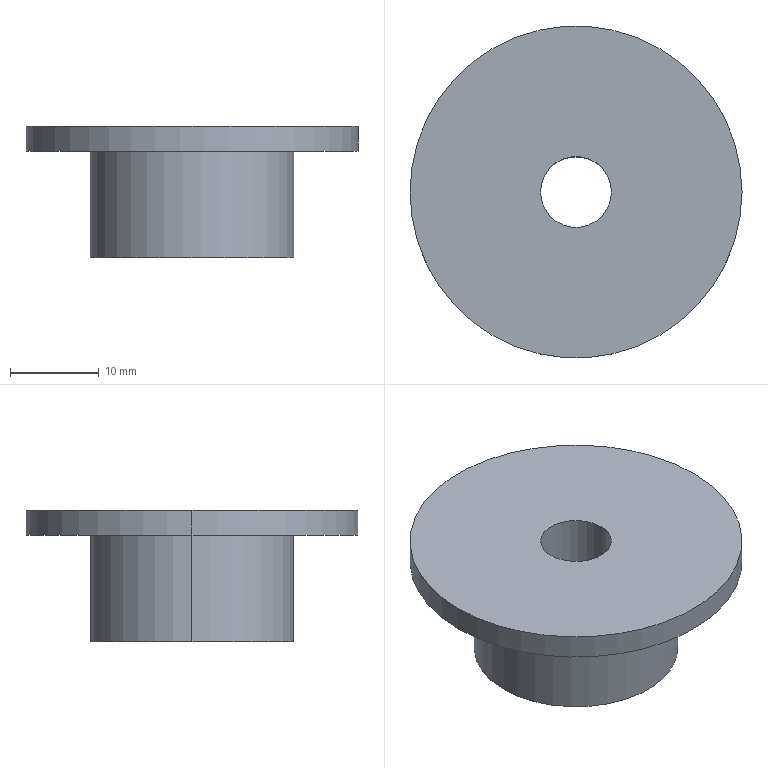Part | SolidWorks | features Extrusion 1, ICE 1 | 1 solid | 9 faces | box 37.5 x 37.5 x 14.8 mm | volume 7334 mm3 | cylinder 6 | plane 3 | commonest cylinder face diameters 8 x2 23 x2 37.5 x2
STEP:
#1=CARTESIAN_POINT('',(18.75,0.,14.8));
#2=VERTEX_POINT('',#1);
#3=CARTESIAN_POINT('',(-18.75,0.,14.8));
#4=VERTEX_POINT('',#3);
#5=CARTESIAN_POINT('',(0.,0.,14.8));
#6=DIRECTION('',(0.,0.,1.));
#7=DIRECTION('',(1.,0.,0.));
#8=AXIS2_PLACEMENT_3D('',#5,#6,#7);
#9=CIRCLE('',#8,18.75);
#10=EDGE_CURVE('',#2,#4,#9,.T.);
#11=ORIENTED_EDGE('',*,*,#10,.F.);
#12=CARTESIAN_POINT('',(18.75,0.,12.));
#13=VERTEX_POINT('',#12);
#14=CARTESIAN_POINT('',(18.75,0.,14.8));
#15=DIRECTION('',(0.,0.,-1.));
#16=VECTOR('',#15,1000.);
#17=LINE('',#14,#16);
#18=EDGE_CURVE('',#2,#13,#17,.T.);
#19=ORIENTED_EDGE('',*,*,#18,.T.);
#20=CARTESIAN_POINT('',(-18.75,0.,12.));
#21=VERTEX_POINT('',#20);
#22=CARTESIAN_POINT('',(0.,0.,12.));
#23=DIRECTION('',(0.,0.,1.));
#24=DIRECTION('',(1.,0.,0.));
#25=AXIS2_PLACEMENT_3D('',#22,#23,#24);
#26=CIRCLE('',#25,18.75);
#27=EDGE_CURVE('',#13,#21,#26,.T.);
#28=ORIENTED_EDGE('',*,*,#27,.T.);
#29=CARTESIAN_POINT('',(-18.75,0.,14.8));
#30=DIRECTION('',(0.,0.,-1.));
#31=VECTOR('',#30,1000.);
#32=LINE('',#29,#31);
#33=EDGE_CURVE('',#4,#21,#32,.T.);
#34=ORIENTED_EDGE('',*,*,#33,.F.);
#35=EDGE_LOOP('',(#11,#19,#28,#34));
#36=FACE_OUTER_BOUND('',#35,.T.);
#37=CARTESIAN_POINT('',(0.,0.,14.8));
#38=DIRECTION('',(0.,0.,-1.));
#39=DIRECTION('',(-1.,0.,0.));
#40=AXIS2_PLACEMENT_3D('',#37,#38,#39);
#41=CYLINDRICAL_SURFACE('',#40,18.75);
#42=ADVANCED_FACE('',(#36),#41,.T.);
#43=CARTESIAN_POINT('',(-4.,0.,14.8));
#44=VERTEX_POINT('',#43);
#45=CARTESIAN_POINT('',(4.,0.,14.8));
#46=VERTEX_POINT('',#45);
#47=CARTESIAN_POINT('',(0.,0.,14.8));
#48=DIRECTION('',(0.,0.,1.));
#49=DIRECTION('',(1.,0.,0.));
#50=AXIS2_PLACEMENT_3D('',#47,#48,#49);
#51=CIRCLE('',#50,4.);
#52=EDGE_CURVE('',#44,#46,#51,.T.);
#53=ORIENTED_EDGE('',*,*,#52,.T.);
#54=CARTESIAN_POINT('',(4.,0.,0.));
#55=VERTEX_POINT('',#54);
#56=CARTESIAN_POINT('',(4.,0.,12.));
#57=DIRECTION('',(0.,0.,-1.));
#58=VECTOR('',#57,1000.);
#59=LINE('',#56,#58);
#60=EDGE_CURVE('',#46,#55,#59,.T.);
#61=ORIENTED_EDGE('',*,*,#60,.T.);
#62=CARTESIAN_POINT('',(-4.,0.,0.));
#63=VERTEX_POINT('',#62);
#64=CARTESIAN_POINT('',(0.,0.,0.));
#65=DIRECTION('',(0.,0.,1.));
#66=DIRECTION('',(1.,0.,0.));
#67=AXIS2_PLACEMENT_3D('',#64,#65,#66);
#68=CIRCLE('',#67,4.);
#69=EDGE_CURVE('',#63,#55,#68,.T.);
#70=ORIENTED_EDGE('',*,*,#69,.F.);
#71=CARTESIAN_POINT('',(-4.,0.,12.));
#72=DIRECTION('',(0.,0.,-1.));
#73=VECTOR('',#72,1000.);
#74=LINE('',#71,#73);
#75=EDGE_CURVE('',#44,#63,#74,.T.);
#76=ORIENTED_EDGE('',*,*,#75,.F.);
#77=EDGE_LOOP('',(#53,#61,#70,#76));
#78=FACE_OUTER_BOUND('',#77,.T.);
#79=CARTESIAN_POINT('',(0.,0.,12.));
#80=DIRECTION('',(0.,0.,-1.));
#81=DIRECTION('',(-1.,0.,0.));
#82=AXIS2_PLACEMENT_3D('',#79,#80,#81);
#83=CYLINDRICAL_SURFACE('',#82,4.);
#84=ADVANCED_FACE('',(#78),#83,.F.);
#85=CARTESIAN_POINT('',(11.5,0.,12.));
#86=VERTEX_POINT('',#85);
#87=CARTESIAN_POINT('',(-11.5,0.,12.));
#88=VERTEX_POINT('',#87);
#89=CARTESIAN_POINT('',(0.,0.,12.));
#90=DIRECTION('',(0.,0.,1.));
#91=DIRECTION('',(1.,0.,0.));
#92=AXIS2_PLACEMENT_3D('',#89,#90,#91);
#93=CIRCLE('',#92,11.5);
#94=EDGE_CURVE('',#86,#88,#93,.T.);
#95=ORIENTED_EDGE('',*,*,#94,.F.);
#96=CARTESIAN_POINT('',(11.5,0.,0.));
#97=VERTEX_POINT('',#96);
#98=CARTESIAN_POINT('',(11.5,0.,12.));
#99=DIRECTION('',(0.,0.,-1.));
#100=VECTOR('',#99,1000.);
#101=LINE('',#98,#100);
#102=EDGE_CURVE('',#86,#97,#101,.T.);
#103=ORIENTED_EDGE('',*,*,#102,.T.);
#104=CARTESIAN_POINT('',(-11.5,0.,0.));
#105=VERTEX_POINT('',#104);
#106=CARTESIAN_POINT('',(0.,0.,0.));
#107=DIRECTION('',(0.,0.,1.));
#108=DIRECTION('',(1.,0.,0.));
#109=AXIS2_PLACEMENT_3D('',#106,#107,#108);
#110=CIRCLE('',#109,11.5);
#111=EDGE_CURVE('',#97,#105,#110,.T.);
#112=ORIENTED_EDGE('',*,*,#111,.T.);
#113=CARTESIAN_POINT('',(-11.5,0.,12.));
#114=DIRECTION('',(0.,0.,-1.));
#115=VECTOR('',#114,1000.);
#116=LINE('',#113,#115);
#117=EDGE_CURVE('',#88,#105,#116,.T.);
#118=ORIENTED_EDGE('',*,*,#117,.F.);
#119=EDGE_LOOP('',(#95,#103,#112,#118));
#120=FACE_OUTER_BOUND('',#119,.T.);
#121=CARTESIAN_POINT('',(0.,0.,12.));
#122=DIRECTION('',(0.,0.,-1.));
#123=DIRECTION('',(-1.,0.,0.));
#124=AXIS2_PLACEMENT_3D('',#121,#122,#123);
#125=CYLINDRICAL_SURFACE('',#124,11.5);
#126=ADVANCED_FACE('',(#120),#125,.T.);
#127=CARTESIAN_POINT('',(0.,0.,0.));
#128=DIRECTION('',(0.,0.,1.));
#129=DIRECTION('',(1.,0.,0.));
#130=AXIS2_PLACEMENT_3D('',#127,#128,#129);
#131=CIRCLE('',#130,11.5);
#132=EDGE_CURVE('',#105,#97,#131,.T.);
#133=ORIENTED_EDGE('',*,*,#132,.F.);
#134=ORIENTED_EDGE('',*,*,#111,.F.);
#135=EDGE_LOOP('',(#133,#134));
#136=FACE_OUTER_BOUND('',#135,.T.);
#137=ORIENTED_EDGE('',*,*,#69,.T.);
#138=CARTESIAN_POINT('',(0.,0.,0.));
#139=DIRECTION('',(0.,0.,1.));
#140=DIRECTION('',(1.,0.,0.));
#141=AXIS2_PLACEMENT_3D('',#138,#139,#140);
#142=CIRCLE('',#141,4.);
#143=EDGE_CURVE('',#55,#63,#142,.T.);
#144=ORIENTED_EDGE('',*,*,#143,.T.);
#145=EDGE_LOOP('',(#137,#144));
#146=FACE_BOUND('',#145,.T.);
#147=CARTESIAN_POINT('',(0.,0.,0.));
#148=DIRECTION('',(0.,0.,1.));
#149=DIRECTION('',(1.,0.,0.));
#150=AXIS2_PLACEMENT_3D('',#147,#148,#149);
#151=PLANE('',#150);
#152=ADVANCED_FACE('',(#136,#146),#151,.F.);
#153=ORIENTED_EDGE('',*,*,#102,.F.);
#154=CARTESIAN_POINT('',(0.,0.,12.));
#155=DIRECTION('',(0.,0.,1.));
#156=DIRECTION('',(1.,0.,0.));
#157=AXIS2_PLACEMENT_3D('',#154,#155,#156);
#158=CIRCLE('',#157,11.5);
#159=EDGE_CURVE('',#88,#86,#158,.T.);
#160=ORIENTED_EDGE('',*,*,#159,.F.);
#161=ORIENTED_EDGE('',*,*,#117,.T.);
#162=ORIENTED_EDGE('',*,*,#132,.T.);
#163=EDGE_LOOP('',(#153,#160,#161,#162));
#164=FACE_OUTER_BOUND('',#163,.T.);
#165=CARTESIAN_POINT('',(0.,0.,12.));
#166=DIRECTION('',(0.,0.,-1.));
#167=DIRECTION('',(-1.,0.,0.));
#168=AXIS2_PLACEMENT_3D('',#165,#166,#167);
#169=CYLINDRICAL_SURFACE('',#168,11.5);
#170=ADVANCED_FACE('',(#164),#169,.T.);
#171=ORIENTED_EDGE('',*,*,#60,.F.);
#172=CARTESIAN_POINT('',(0.,0.,14.8));
#173=DIRECTION('',(0.,0.,1.));
#174=DIRECTION('',(1.,0.,0.));
#175=AXIS2_PLACEMENT_3D('',#172,#173,#174);
#176=CIRCLE('',#175,4.);
#177=EDGE_CURVE('',#46,#44,#176,.T.);
#178=ORIENTED_EDGE('',*,*,#177,.T.);
#179=ORIENTED_EDGE('',*,*,#75,.T.);
#180=ORIENTED_EDGE('',*,*,#143,.F.);
#181=EDGE_LOOP('',(#171,#178,#179,#180));
#182=FACE_OUTER_BOUND('',#181,.T.);
#183=CARTESIAN_POINT('',(0.,0.,12.));
#184=DIRECTION('',(0.,0.,-1.));
#185=DIRECTION('',(-1.,0.,0.));
#186=AXIS2_PLACEMENT_3D('',#183,#184,#185);
#187=CYLINDRICAL_SURFACE('',#186,4.);
#188=ADVANCED_FACE('',(#182),#187,.F.);
#189=CARTESIAN_POINT('',(0.,0.,12.));
#190=DIRECTION('',(0.,0.,1.));
#191=DIRECTION('',(1.,0.,0.));
#192=AXIS2_PLACEMENT_3D('',#189,#190,#191);
#193=CIRCLE('',#192,18.75);
#194=EDGE_CURVE('',#21,#13,#193,.T.);
#195=ORIENTED_EDGE('',*,*,#194,.F.);
#196=ORIENTED_EDGE('',*,*,#27,.F.);
#197=EDGE_LOOP('',(#195,#196));
#198=FACE_OUTER_BOUND('',#197,.T.);
#199=ORIENTED_EDGE('',*,*,#159,.T.);
#200=ORIENTED_EDGE('',*,*,#94,.T.);
#201=EDGE_LOOP('',(#199,#200));
#202=FACE_BOUND('',#201,.T.);
#203=CARTESIAN_POINT('',(0.,0.,12.));
#204=DIRECTION('',(0.,0.,1.));
#205=DIRECTION('',(1.,0.,0.));
#206=AXIS2_PLACEMENT_3D('',#203,#204,#205);
#207=PLANE('',#206);
#208=ADVANCED_FACE('',(#198,#202),#207,.F.);
#209=CARTESIAN_POINT('',(0.,0.,14.8));
#210=DIRECTION('',(0.,0.,1.));
#211=DIRECTION('',(1.,0.,0.));
#212=AXIS2_PLACEMENT_3D('',#209,#210,#211);
#213=CIRCLE('',#212,18.75);
#214=EDGE_CURVE('',#4,#2,#213,.T.);
#215=ORIENTED_EDGE('',*,*,#214,.T.);
#216=ORIENTED_EDGE('',*,*,#10,.T.);
#217=EDGE_LOOP('',(#215,#216));
#218=FACE_OUTER_BOUND('',#217,.T.);
#219=ORIENTED_EDGE('',*,*,#52,.F.);
#220=ORIENTED_EDGE('',*,*,#177,.F.);
#221=EDGE_LOOP('',(#219,#220));
#222=FACE_BOUND('',#221,.T.);
#223=CARTESIAN_POINT('',(0.,0.,14.8));
#224=DIRECTION('',(0.,0.,1.));
#225=DIRECTION('',(1.,0.,0.));
#226=AXIS2_PLACEMENT_3D('',#223,#224,#225);
#227=PLANE('',#226);
#228=ADVANCED_FACE('',(#218,#222),#227,.T.);
#229=ORIENTED_EDGE('',*,*,#18,.F.);
#230=ORIENTED_EDGE('',*,*,#214,.F.);
#231=ORIENTED_EDGE('',*,*,#33,.T.);
#232=ORIENTED_EDGE('',*,*,#194,.T.);
#233=EDGE_LOOP('',(#229,#230,#231,#232));
#234=FACE_OUTER_BOUND('',#233,.T.);
#235=CARTESIAN_POINT('',(0.,0.,14.8));
#236=DIRECTION('',(0.,0.,-1.));
#237=DIRECTION('',(-1.,0.,0.));
#238=AXIS2_PLACEMENT_3D('',#235,#236,#237);
#239=CYLINDRICAL_SURFACE('',#238,18.75);
#240=ADVANCED_FACE('',(#234),#239,.T.);
#241=CLOSED_SHELL('',(#42,#84,#126,#152,#170,#188,#208,#228,#240));
#242=MANIFOLD_SOLID_BREP('',#241);
#243=CARTESIAN_POINT('',(0.,0.,0.));
#244=DIRECTION('',(0.,0.,1.));
#245=DIRECTION('',(1.,0.,0.));
#246=AXIS2_PLACEMENT_3D('',#243,#244,#245);
#247=(LENGTH_UNIT()NAMED_UNIT(*)SI_UNIT(.MILLI.,.METRE.));
#248=UNCERTAINTY_MEASURE_WITH_UNIT(LENGTH_MEASURE(0.00001),#247,'','');
#249=(NAMED_UNIT(*)PLANE_ANGLE_UNIT()SI_UNIT($,.RADIAN.));
#250=(NAMED_UNIT(*)SI_UNIT($,.STERADIAN.)SOLID_ANGLE_UNIT());
#251=(GEOMETRIC_REPRESENTATION_CONTEXT(3)GLOBAL_UNCERTAINTY_ASSIGNED_CONTEXT((#248))GLOBAL_UNIT_ASSIGNED_CONTEXT((#247,#249,#250))REPRESENTATION_CONTEXT('',''));
#252=ADVANCED_BREP_SHAPE_REPRESENTATION('',(#242,#246),#251);